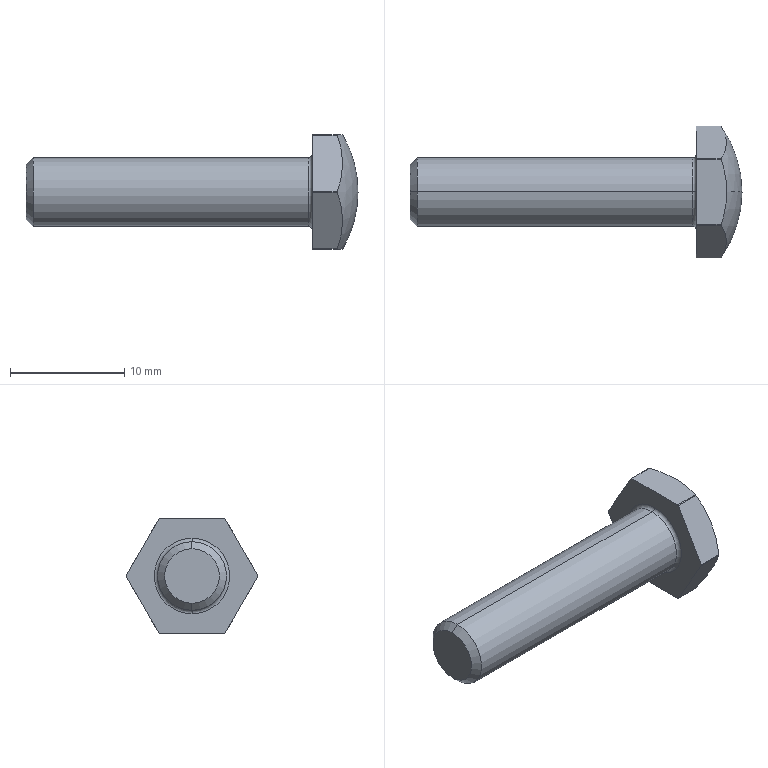Part | STEP file | SSTBB6-25-Part-1-2 | 1 solid | 22 faces | box 29 x 11.5 x 10 mm | volume 987.027 mm3 | cylinder 8 | plane 8 | cone 2 | torus 2 | sphere 2 | commonest cylinder face diameters 11.5 x6 6 x2
STEP:
#1=CARTESIAN_POINT('',(-5.,0.,2.387));
#2=VERTEX_POINT('',#1);
#3=CARTESIAN_POINT('',(-5.,0.,-2.387));
#4=VERTEX_POINT('',#3);
#5=CARTESIAN_POINT('',(-5.,0.,0.));
#6=DIRECTION('',(-1.,0.,0.));
#7=DIRECTION('',(0.,0.,1.));
#8=AXIS2_PLACEMENT_3D('',#5,#6,#7);
#9=CIRCLE('',#8,2.387);
#10=EDGE_CURVE('',#2,#4,#9,.T.);
#11=ORIENTED_EDGE('',*,*,#10,.F.);
#12=CARTESIAN_POINT('',(-4.386,0.,3.));
#13=VERTEX_POINT('',#12);
#14=CARTESIAN_POINT('',(-4.386,0.,3.));
#15=DIRECTION('',(0.7071,0.,0.7071));
#16=VECTOR('',#15,1000.);
#17=LINE('',#14,#16);
#18=EDGE_CURVE('',#2,#13,#17,.T.);
#19=ORIENTED_EDGE('',*,*,#18,.T.);
#20=CARTESIAN_POINT('',(-4.386,0.,-3.));
#21=VERTEX_POINT('',#20);
#22=CARTESIAN_POINT('',(-4.386,0.,0.));
#23=DIRECTION('',(-1.,0.,0.));
#24=DIRECTION('',(0.,0.,1.));
#25=AXIS2_PLACEMENT_3D('',#22,#23,#24);
#26=CIRCLE('',#25,3.);
#27=EDGE_CURVE('',#13,#21,#26,.T.);
#28=ORIENTED_EDGE('',*,*,#27,.T.);
#29=CARTESIAN_POINT('',(-4.386,0.,-3.));
#30=DIRECTION('',(0.7071,0.,-0.7071));
#31=VECTOR('',#30,1000.);
#32=LINE('',#29,#31);
#33=EDGE_CURVE('',#4,#21,#32,.T.);
#34=ORIENTED_EDGE('',*,*,#33,.F.);
#35=EDGE_LOOP('',(#11,#19,#28,#34));
#36=FACE_OUTER_BOUND('',#35,.T.);
#37=CARTESIAN_POINT('',(-4.386,0.,0.));
#38=DIRECTION('',(1.,0.,0.));
#39=DIRECTION('',(0.,0.,-1.));
#40=AXIS2_PLACEMENT_3D('',#37,#38,#39);
#41=CONICAL_SURFACE('',#40,3.,0.7854);
#42=ADVANCED_FACE('',(#36),#41,.T.);
#43=CARTESIAN_POINT('',(19.7,0.,3.));
#44=VERTEX_POINT('',#43);
#45=CARTESIAN_POINT('',(19.7,0.,-3.));
#46=VERTEX_POINT('',#45);
#47=CARTESIAN_POINT('',(19.7,0.,0.));
#48=DIRECTION('',(-1.,0.,0.));
#49=DIRECTION('',(0.,0.,1.));
#50=AXIS2_PLACEMENT_3D('',#47,#48,#49);
#51=CIRCLE('',#50,3.);
#52=EDGE_CURVE('',#44,#46,#51,.T.);
#53=ORIENTED_EDGE('',*,*,#52,.T.);
#54=CARTESIAN_POINT('',(0.,0.,-3.));
#55=DIRECTION('',(-1.,0.,0.));
#56=VECTOR('',#55,1000.);
#57=LINE('',#54,#56);
#58=EDGE_CURVE('',#46,#21,#57,.T.);
#59=ORIENTED_EDGE('',*,*,#58,.T.);
#60=ORIENTED_EDGE('',*,*,#27,.F.);
#61=CARTESIAN_POINT('',(0.,0.,3.));
#62=DIRECTION('',(-1.,0.,0.));
#63=VECTOR('',#62,1000.);
#64=LINE('',#61,#63);
#65=EDGE_CURVE('',#44,#13,#64,.T.);
#66=ORIENTED_EDGE('',*,*,#65,.F.);
#67=EDGE_LOOP('',(#53,#59,#60,#66));
#68=FACE_OUTER_BOUND('',#67,.T.);
#69=CARTESIAN_POINT('',(0.,0.,0.));
#70=DIRECTION('',(-1.,0.,0.));
#71=DIRECTION('',(0.,0.,1.));
#72=AXIS2_PLACEMENT_3D('',#69,#70,#71);
#73=CYLINDRICAL_SURFACE('',#72,3.);
#74=ADVANCED_FACE('',(#68),#73,.T.);
#75=CARTESIAN_POINT('',(19.7,0.,0.));
#76=DIRECTION('',(-1.,0.,0.));
#77=DIRECTION('',(0.,0.,1.));
#78=AXIS2_PLACEMENT_3D('',#75,#76,#77);
#79=CIRCLE('',#78,3.);
#80=EDGE_CURVE('',#46,#44,#79,.T.);
#81=ORIENTED_EDGE('',*,*,#80,.F.);
#82=CARTESIAN_POINT('',(20.,0.,-3.3));
#83=VERTEX_POINT('',#82);
#84=CARTESIAN_POINT('',(19.7,0.,-3.3));
#85=DIRECTION('',(0.,1.,0.));
#86=DIRECTION('',(0.,0.,1.));
#87=AXIS2_PLACEMENT_3D('',#84,#85,#86);
#88=CIRCLE('',#87,0.3);
#89=EDGE_CURVE('',#46,#83,#88,.T.);
#90=ORIENTED_EDGE('',*,*,#89,.T.);
#91=CARTESIAN_POINT('',(20.,0.,3.3));
#92=VERTEX_POINT('',#91);
#93=CARTESIAN_POINT('',(20.,0.,0.));
#94=DIRECTION('',(-1.,0.,0.));
#95=DIRECTION('',(0.,0.,1.));
#96=AXIS2_PLACEMENT_3D('',#93,#94,#95);
#97=CIRCLE('',#96,3.3);
#98=EDGE_CURVE('',#83,#92,#97,.T.);
#99=ORIENTED_EDGE('',*,*,#98,.T.);
#100=CARTESIAN_POINT('',(19.7,0.,3.3));
#101=DIRECTION('',(0.,-1.,0.));
#102=DIRECTION('',(0.,0.,-1.));
#103=AXIS2_PLACEMENT_3D('',#100,#101,#102);
#104=CIRCLE('',#103,0.3);
#105=EDGE_CURVE('',#44,#92,#104,.T.);
#106=ORIENTED_EDGE('',*,*,#105,.F.);
#107=EDGE_LOOP('',(#81,#90,#99,#106));
#108=FACE_OUTER_BOUND('',#107,.T.);
#109=CARTESIAN_POINT('',(19.7,0.,0.));
#110=DIRECTION('',(-1.,0.,0.));
#111=DIRECTION('',(0.,0.,1.));
#112=AXIS2_PLACEMENT_3D('',#109,#110,#111);
#113=TOROIDAL_SURFACE('',#112,3.3,0.3);
#114=ADVANCED_FACE('',(#108),#113,.F.);
#115=CARTESIAN_POINT('',(24.,0.,0.));
#116=VERTEX_POINT('',#115);
#117=CARTESIAN_POINT('',(22.66,0.,5.));
#118=VERTEX_POINT('',#117);
#119=CARTESIAN_POINT('',(14.,0.,0.));
#120=DIRECTION('',(0.,-1.,0.));
#121=DIRECTION('',(0.,0.,-1.));
#122=AXIS2_PLACEMENT_3D('',#119,#120,#121);
#123=CIRCLE('',#122,10.);
#124=EDGE_CURVE('',#116,#118,#123,.T.);
#125=ORIENTED_EDGE('',*,*,#124,.F.);
#126=CARTESIAN_POINT('',(22.66,0.,-5.));
#127=VERTEX_POINT('',#126);
#128=CARTESIAN_POINT('',(14.,0.,0.));
#129=DIRECTION('',(0.,1.,0.));
#130=DIRECTION('',(0.,0.,1.));
#131=AXIS2_PLACEMENT_3D('',#128,#129,#130);
#132=CIRCLE('',#131,10.);
#133=EDGE_CURVE('',#116,#127,#132,.T.);
#134=ORIENTED_EDGE('',*,*,#133,.T.);
#135=CARTESIAN_POINT('',(22.182,2.839,-5.));
#136=VERTEX_POINT('',#135);
#137=CARTESIAN_POINT('',(14.,0.,-5.));
#138=DIRECTION('',(0.,0.,1.));
#139=DIRECTION('',(-1.,0.,0.));
#140=AXIS2_PLACEMENT_3D('',#137,#138,#139);
#141=CIRCLE('',#140,8.66);
#142=EDGE_CURVE('',#127,#136,#141,.T.);
#143=ORIENTED_EDGE('',*,*,#142,.T.);
#144=CARTESIAN_POINT('',(22.182,2.91,-4.959));
#145=VERTEX_POINT('',#144);
#146=CARTESIAN_POINT('',(22.182,0.,0.));
#147=DIRECTION('',(-1.,0.,0.));
#148=DIRECTION('',(0.,0.,1.));
#149=AXIS2_PLACEMENT_3D('',#146,#147,#148);
#150=CIRCLE('',#149,5.75);
#151=EDGE_CURVE('',#145,#136,#150,.T.);
#152=ORIENTED_EDGE('',*,*,#151,.F.);
#153=CARTESIAN_POINT('',(22.182,5.75,-0.04096));
#154=VERTEX_POINT('',#153);
#155=CARTESIAN_POINT('',(14.,4.33,-2.5));
#156=DIRECTION('',(0.,-0.866,0.5));
#157=DIRECTION('',(0.,-0.5,-0.866));
#158=AXIS2_PLACEMENT_3D('',#155,#156,#157);
#159=CIRCLE('',#158,8.66);
#160=EDGE_CURVE('',#145,#154,#159,.T.);
#161=ORIENTED_EDGE('',*,*,#160,.T.);
#162=CARTESIAN_POINT('',(22.182,5.75,0.04096));
#163=VERTEX_POINT('',#162);
#164=CARTESIAN_POINT('',(22.182,0.,0.));
#165=DIRECTION('',(-1.,0.,0.));
#166=DIRECTION('',(0.,0.,1.));
#167=AXIS2_PLACEMENT_3D('',#164,#165,#166);
#168=CIRCLE('',#167,5.75);
#169=EDGE_CURVE('',#163,#154,#168,.T.);
#170=ORIENTED_EDGE('',*,*,#169,.F.);
#171=CARTESIAN_POINT('',(22.182,2.91,4.959));
#172=VERTEX_POINT('',#171);
#173=CARTESIAN_POINT('',(14.,4.33,2.5));
#174=DIRECTION('',(0.,-0.866,-0.5));
#175=DIRECTION('',(0.,0.5,-0.866));
#176=AXIS2_PLACEMENT_3D('',#173,#174,#175);
#177=CIRCLE('',#176,8.66);
#178=EDGE_CURVE('',#163,#172,#177,.T.);
#179=ORIENTED_EDGE('',*,*,#178,.T.);
#180=CARTESIAN_POINT('',(22.182,2.839,5.));
#181=VERTEX_POINT('',#180);
#182=CARTESIAN_POINT('',(22.182,0.,0.));
#183=DIRECTION('',(-1.,0.,0.));
#184=DIRECTION('',(0.,0.,1.));
#185=AXIS2_PLACEMENT_3D('',#182,#183,#184);
#186=CIRCLE('',#185,5.75);
#187=EDGE_CURVE('',#181,#172,#186,.T.);
#188=ORIENTED_EDGE('',*,*,#187,.F.);
#189=CARTESIAN_POINT('',(14.,0.,5.));
#190=DIRECTION('',(0.,0.,-1.));
#191=DIRECTION('',(1.,0.,0.));
#192=AXIS2_PLACEMENT_3D('',#189,#190,#191);
#193=CIRCLE('',#192,8.66);
#194=EDGE_CURVE('',#181,#118,#193,.T.);
#195=ORIENTED_EDGE('',*,*,#194,.T.);
#196=EDGE_LOOP('',(#125,#134,#143,#152,#161,#170,#179,#188,#195));
#197=FACE_OUTER_BOUND('',#196,.T.);
#198=CARTESIAN_POINT('',(14.,0.,0.));
#199=DIRECTION('',(0.,1.,0.));
#200=DIRECTION('',(0.,0.,1.));
#201=AXIS2_PLACEMENT_3D('',#198,#199,#200);
#202=SPHERICAL_SURFACE('',#201,10.);
#203=ADVANCED_FACE('',(#197),#202,.T.);
#204=ORIENTED_EDGE('',*,*,#133,.F.);
#205=ORIENTED_EDGE('',*,*,#124,.T.);
#206=CARTESIAN_POINT('',(22.182,-2.839,5.));
#207=VERTEX_POINT('',#206);
#208=CARTESIAN_POINT('',(14.,0.,5.));
#209=DIRECTION('',(0.,0.,-1.));
#210=DIRECTION('',(1.,0.,0.));
#211=AXIS2_PLACEMENT_3D('',#208,#209,#210);
#212=CIRCLE('',#211,8.66);
#213=EDGE_CURVE('',#118,#207,#212,.T.);
#214=ORIENTED_EDGE('',*,*,#213,.T.);
#215=CARTESIAN_POINT('',(22.182,-2.91,4.959));
#216=VERTEX_POINT('',#215);
#217=CARTESIAN_POINT('',(22.182,0.,0.));
#218=DIRECTION('',(-1.,0.,0.));
#219=DIRECTION('',(0.,0.,1.));
#220=AXIS2_PLACEMENT_3D('',#217,#218,#219);
#221=CIRCLE('',#220,5.75);
#222=EDGE_CURVE('',#216,#207,#221,.T.);
#223=ORIENTED_EDGE('',*,*,#222,.F.);
#224=CARTESIAN_POINT('',(22.182,-5.75,0.04096));
#225=VERTEX_POINT('',#224);
#226=CARTESIAN_POINT('',(14.,-4.33,2.5));
#227=DIRECTION('',(0.,0.866,-0.5));
#228=DIRECTION('',(0.,0.5,0.866));
#229=AXIS2_PLACEMENT_3D('',#226,#227,#228);
#230=CIRCLE('',#229,8.66);
#231=EDGE_CURVE('',#216,#225,#230,.T.);
#232=ORIENTED_EDGE('',*,*,#231,.T.);
#233=CARTESIAN_POINT('',(22.182,-5.75,-0.04096));
#234=VERTEX_POINT('',#233);
#235=CARTESIAN_POINT('',(22.182,0.,0.));
#236=DIRECTION('',(-1.,0.,0.));
#237=DIRECTION('',(0.,0.,1.));
#238=AXIS2_PLACEMENT_3D('',#235,#236,#237);
#239=CIRCLE('',#238,5.75);
#240=EDGE_CURVE('',#234,#225,#239,.T.);
#241=ORIENTED_EDGE('',*,*,#240,.F.);
#242=CARTESIAN_POINT('',(22.182,-2.91,-4.959));
#243=VERTEX_POINT('',#242);
#244=CARTESIAN_POINT('',(14.,-4.33,-2.5));
#245=DIRECTION('',(0.,0.866,0.5));
#246=DIRECTION('',(0.,-0.5,0.866));
#247=AXIS2_PLACEMENT_3D('',#244,#245,#246);
#248=CIRCLE('',#247,8.66);
#249=EDGE_CURVE('',#234,#243,#248,.T.);
#250=ORIENTED_EDGE('',*,*,#249,.T.);
#251=CARTESIAN_POINT('',(22.182,-2.839,-5.));
#252=VERTEX_POINT('',#251);
#253=CARTESIAN_POINT('',(22.182,0.,0.));
#254=DIRECTION('',(-1.,0.,0.));
#255=DIRECTION('',(0.,0.,1.));
#256=AXIS2_PLACEMENT_3D('',#253,#254,#255);
#257=CIRCLE('',#256,5.75);
#258=EDGE_CURVE('',#252,#243,#257,.T.);
#259=ORIENTED_EDGE('',*,*,#258,.F.);
#260=CARTESIAN_POINT('',(14.,0.,-5.));
#261=DIRECTION('',(0.,0.,1.));
#262=DIRECTION('',(-1.,0.,0.));
#263=AXIS2_PLACEMENT_3D('',#260,#261,#262);
#264=CIRCLE('',#263,8.66);
#265=EDGE_CURVE('',#252,#127,#264,.T.);
#266=ORIENTED_EDGE('',*,*,#265,.T.);
#267=EDGE_LOOP('',(#204,#205,#214,#223,#232,#241,#250,#259,#266));
#268=FACE_OUTER_BOUND('',#267,.T.);
#269=CARTESIAN_POINT('',(14.,0.,0.));
#270=DIRECTION('',(0.,1.,0.));
#271=DIRECTION('',(0.,0.,1.));
#272=AXIS2_PLACEMENT_3D('',#269,#270,#271);
#273=SPHERICAL_SURFACE('',#272,10.);
#274=ADVANCED_FACE('',(#268),#273,.T.);
#275=CARTESIAN_POINT('',(20.,-2.839,-5.));
#276=VERTEX_POINT('',#275);
#277=CARTESIAN_POINT('',(0.,-2.839,-5.));
#278=DIRECTION('',(-1.,0.,0.));
#279=VECTOR('',#278,1000.);
#280=LINE('',#277,#279);
#281=EDGE_CURVE('',#252,#276,#280,.T.);
#282=ORIENTED_EDGE('',*,*,#281,.F.);
#283=ORIENTED_EDGE('',*,*,#258,.T.);
#284=CARTESIAN_POINT('',(20.,-2.91,-4.959));
#285=VERTEX_POINT('',#284);
#286=CARTESIAN_POINT('',(0.,-2.91,-4.959));
#287=DIRECTION('',(1.,0.,0.));
#288=VECTOR('',#287,1000.);
#289=LINE('',#286,#288);
#290=EDGE_CURVE('',#285,#243,#289,.T.);
#291=ORIENTED_EDGE('',*,*,#290,.F.);
#292=CARTESIAN_POINT('',(20.,0.,0.));
#293=DIRECTION('',(-1.,0.,0.));
#294=DIRECTION('',(0.,0.,1.));
#295=AXIS2_PLACEMENT_3D('',#292,#293,#294);
#296=CIRCLE('',#295,5.75);
#297=EDGE_CURVE('',#276,#285,#296,.T.);
#298=ORIENTED_EDGE('',*,*,#297,.F.);
#299=EDGE_LOOP('',(#282,#283,#291,#298));
#300=FACE_OUTER_BOUND('',#299,.T.);
#301=CARTESIAN_POINT('',(0.,0.,0.));
#302=DIRECTION('',(-1.,0.,0.));
#303=DIRECTION('',(0.,0.,1.));
#304=AXIS2_PLACEMENT_3D('',#301,#302,#303);
#305=CYLINDRICAL_SURFACE('',#304,5.75);
#306=ADVANCED_FACE('',(#300),#305,.T.);
#307=CARTESIAN_POINT('',(20.,2.839,-5.));
#308=VERTEX_POINT('',#307);
#309=CARTESIAN_POINT('',(0.,2.839,-5.));
#310=DIRECTION('',(1.,0.,0.));
#311=VECTOR('',#310,1000.);
#312=LINE('',#309,#311);
#313=EDGE_CURVE('',#308,#136,#312,.T.);
#314=ORIENTED_EDGE('',*,*,#313,.F.);
#315=CARTESIAN_POINT('',(20.,2.91,-4.959));
#316=VERTEX_POINT('',#315);
#317=CARTESIAN_POINT('',(20.,0.,0.));
#318=DIRECTION('',(-1.,0.,0.));
#319=DIRECTION('',(0.,0.,1.));
#320=AXIS2_PLACEMENT_3D('',#317,#318,#319);
#321=CIRCLE('',#320,5.75);
#322=EDGE_CURVE('',#316,#308,#321,.T.);
#323=ORIENTED_EDGE('',*,*,#322,.F.);
#324=CARTESIAN_POINT('',(0.,2.91,-4.959));
#325=DIRECTION('',(-1.,0.,0.));
#326=VECTOR('',#325,1000.);
#327=LINE('',#324,#326);
#328=EDGE_CURVE('',#145,#316,#327,.T.);
#329=ORIENTED_EDGE('',*,*,#328,.F.);
#330=ORIENTED_EDGE('',*,*,#151,.T.);
#331=EDGE_LOOP('',(#314,#323,#329,#330));
#332=FACE_OUTER_BOUND('',#331,.T.);
#333=CARTESIAN_POINT('',(0.,0.,0.));
#334=DIRECTION('',(-1.,0.,0.));
#335=DIRECTION('',(0.,0.,1.));
#336=AXIS2_PLACEMENT_3D('',#333,#334,#335);
#337=CYLINDRICAL_SURFACE('',#336,5.75);
#338=ADVANCED_FACE('',(#332),#337,.T.);
#339=CARTESIAN_POINT('',(20.,5.75,-0.04096));
#340=VERTEX_POINT('',#339);
#341=CARTESIAN_POINT('',(0.,5.75,-0.04096));
#342=DIRECTION('',(1.,0.,0.));
#343=VECTOR('',#342,1000.);
#344=LINE('',#341,#343);
#345=EDGE_CURVE('',#340,#154,#344,.T.);
#346=ORIENTED_EDGE('',*,*,#345,.F.);
#347=CARTESIAN_POINT('',(20.,5.75,0.04096));
#348=VERTEX_POINT('',#347);
#349=CARTESIAN_POINT('',(20.,0.,0.));
#350=DIRECTION('',(-1.,0.,0.));
#351=DIRECTION('',(0.,0.,1.));
#352=AXIS2_PLACEMENT_3D('',#349,#350,#351);
#353=CIRCLE('',#352,5.75);
#354=EDGE_CURVE('',#348,#340,#353,.T.);
#355=ORIENTED_EDGE('',*,*,#354,.F.);
#356=CARTESIAN_POINT('',(0.,5.75,0.04096));
#357=DIRECTION('',(-1.,0.,0.));
#358=VECTOR('',#357,1000.);
#359=LINE('',#356,#358);
#360=EDGE_CURVE('',#163,#348,#359,.T.);
#361=ORIENTED_EDGE('',*,*,#360,.F.);
#362=ORIENTED_EDGE('',*,*,#169,.T.);
#363=EDGE_LOOP('',(#346,#355,#361,#362));
#364=FACE_OUTER_BOUND('',#363,.T.);
#365=CARTESIAN_POINT('',(0.,0.,0.));
#366=DIRECTION('',(-1.,0.,0.));
#367=DIRECTION('',(0.,0.,1.));
#368=AXIS2_PLACEMENT_3D('',#365,#366,#367);
#369=CYLINDRICAL_SURFACE('',#368,5.75);
#370=ADVANCED_FACE('',(#364),#369,.T.);
#371=CARTESIAN_POINT('',(20.,2.91,4.959));
#372=VERTEX_POINT('',#371);
#373=CARTESIAN_POINT('',(0.,2.91,4.959));
#374=DIRECTION('',(1.,0.,0.));
#375=VECTOR('',#374,1000.);
#376=LINE('',#373,#375);
#377=EDGE_CURVE('',#372,#172,#376,.T.);
#378=ORIENTED_EDGE('',*,*,#377,.F.);
#379=CARTESIAN_POINT('',(20.,2.839,5.));
#380=VERTEX_POINT('',#379);
#381=CARTESIAN_POINT('',(20.,0.,0.));
#382=DIRECTION('',(-1.,0.,0.));
#383=DIRECTION('',(0.,0.,1.));
#384=AXIS2_PLACEMENT_3D('',#381,#382,#383);
#385=CIRCLE('',#384,5.75);
#386=EDGE_CURVE('',#380,#372,#385,.T.);
#387=ORIENTED_EDGE('',*,*,#386,.F.);
#388=CARTESIAN_POINT('',(0.,2.839,5.));
#389=DIRECTION('',(-1.,0.,0.));
#390=VECTOR('',#389,1000.);
#391=LINE('',#388,#390);
#392=EDGE_CURVE('',#181,#380,#391,.T.);
#393=ORIENTED_EDGE('',*,*,#392,.F.);
#394=ORIENTED_EDGE('',*,*,#187,.T.);
#395=EDGE_LOOP('',(#378,#387,#393,#394));
#396=FACE_OUTER_BOUND('',#395,.T.);
#397=CARTESIAN_POINT('',(0.,0.,0.));
#398=DIRECTION('',(-1.,0.,0.));
#399=DIRECTION('',(0.,0.,1.));
#400=AXIS2_PLACEMENT_3D('',#397,#398,#399);
#401=CYLINDRICAL_SURFACE('',#400,5.75);
#402=ADVANCED_FACE('',(#396),#401,.T.);
#403=CARTESIAN_POINT('',(20.,-2.839,5.));
#404=VERTEX_POINT('',#403);
#405=CARTESIAN_POINT('',(0.,-2.839,5.));
#406=DIRECTION('',(1.,0.,0.));
#407=VECTOR('',#406,1000.);
#408=LINE('',#405,#407);
#409=EDGE_CURVE('',#404,#207,#408,.T.);
#410=ORIENTED_EDGE('',*,*,#409,.F.);
#411=CARTESIAN_POINT('',(20.,-2.91,4.959));
#412=VERTEX_POINT('',#411);
#413=CARTESIAN_POINT('',(20.,0.,0.));
#414=DIRECTION('',(-1.,0.,0.));
#415=DIRECTION('',(0.,0.,1.));
#416=AXIS2_PLACEMENT_3D('',#413,#414,#415);
#417=CIRCLE('',#416,5.75);
#418=EDGE_CURVE('',#412,#404,#417,.T.);
#419=ORIENTED_EDGE('',*,*,#418,.F.);
#420=CARTESIAN_POINT('',(0.,-2.91,4.959));
#421=DIRECTION('',(-1.,0.,0.));
#422=VECTOR('',#421,1000.);
#423=LINE('',#420,#422);
#424=EDGE_CURVE('',#216,#412,#423,.T.);
#425=ORIENTED_EDGE('',*,*,#424,.F.);
#426=ORIENTED_EDGE('',*,*,#222,.T.);
#427=EDGE_LOOP('',(#410,#419,#425,#426));
#428=FACE_OUTER_BOUND('',#427,.T.);
#429=CARTESIAN_POINT('',(0.,0.,0.));
#430=DIRECTION('',(-1.,0.,0.));
#431=DIRECTION('',(0.,0.,1.));
#432=AXIS2_PLACEMENT_3D('',#429,#430,#431);
#433=CYLINDRICAL_SURFACE('',#432,5.75);
#434=ADVANCED_FACE('',(#428),#433,.T.);
#435=CARTESIAN_POINT('',(20.,-5.75,0.04096));
#436=VERTEX_POINT('',#435);
#437=CARTESIAN_POINT('',(0.,-5.75,0.04096));
#438=DIRECTION('',(1.,0.,0.));
#439=VECTOR('',#438,1000.);
#440=LINE('',#437,#439);
#441=EDGE_CURVE('',#436,#225,#440,.T.);
#442=ORIENTED_EDGE('',*,*,#441,.F.);
#443=CARTESIAN_POINT('',(20.,-5.75,-0.04096));
#444=VERTEX_POINT('',#443);
#445=CARTESIAN_POINT('',(20.,0.,0.));
#446=DIRECTION('',(-1.,0.,0.));
#447=DIRECTION('',(0.,0.,1.));
#448=AXIS2_PLACEMENT_3D('',#445,#446,#447);
#449=CIRCLE('',#448,5.75);
#450=EDGE_CURVE('',#444,#436,#449,.T.);
#451=ORIENTED_EDGE('',*,*,#450,.F.);
#452=CARTESIAN_POINT('',(0.,-5.75,-0.04096));
#453=DIRECTION('',(-1.,0.,0.));
#454=VECTOR('',#453,1000.);
#455=LINE('',#452,#454);
#456=EDGE_CURVE('',#234,#444,#455,.T.);
#457=ORIENTED_EDGE('',*,*,#456,.F.);
#458=ORIENTED_EDGE('',*,*,#240,.T.);
#459=EDGE_LOOP('',(#442,#451,#457,#458));
#460=FACE_OUTER_BOUND('',#459,.T.);
#461=CARTESIAN_POINT('',(0.,0.,0.));
#462=DIRECTION('',(-1.,0.,0.));
#463=DIRECTION('',(0.,0.,1.));
#464=AXIS2_PLACEMENT_3D('',#461,#462,#463);
#465=CYLINDRICAL_SURFACE('',#464,5.75);
#466=ADVANCED_FACE('',(#460),#465,.T.);
#467=CARTESIAN_POINT('',(20.,0.,0.));
#468=DIRECTION('',(-1.,0.,0.));
#469=DIRECTION('',(0.,0.,1.));
#470=AXIS2_PLACEMENT_3D('',#467,#468,#469);
#471=CIRCLE('',#470,3.3);
#472=EDGE_CURVE('',#92,#83,#471,.T.);
#473=ORIENTED_EDGE('',*,*,#472,.F.);
#474=ORIENTED_EDGE('',*,*,#98,.F.);
#475=EDGE_LOOP('',(#473,#474));
#476=FACE_BOUND('',#475,.T.);
#477=CARTESIAN_POINT('',(20.,0.,-5.));
#478=DIRECTION('',(0.,1.,0.));
#479=VECTOR('',#478,1000.);
#480=LINE('',#477,#479);
#481=EDGE_CURVE('',#276,#308,#480,.T.);
#482=ORIENTED_EDGE('',*,*,#481,.F.);
#483=ORIENTED_EDGE('',*,*,#297,.T.);
#484=CARTESIAN_POINT('',(20.,-6.82,1.812));
#485=DIRECTION('',(0.,0.5,-0.866));
#486=VECTOR('',#485,1000.);
#487=LINE('',#484,#486);
#488=EDGE_CURVE('',#444,#285,#487,.T.);
#489=ORIENTED_EDGE('',*,*,#488,.F.);
#490=ORIENTED_EDGE('',*,*,#450,.T.);
#491=CARTESIAN_POINT('',(20.,-1.84,6.812));
#492=DIRECTION('',(0.,-0.5,-0.866));
#493=VECTOR('',#492,1000.);
#494=LINE('',#491,#493);
#495=EDGE_CURVE('',#412,#436,#494,.T.);
#496=ORIENTED_EDGE('',*,*,#495,.F.);
#497=ORIENTED_EDGE('',*,*,#418,.T.);
#498=CARTESIAN_POINT('',(20.,0.,5.));
#499=DIRECTION('',(0.,-1.,0.));
#500=VECTOR('',#499,1000.);
#501=LINE('',#498,#500);
#502=EDGE_CURVE('',#380,#404,#501,.T.);
#503=ORIENTED_EDGE('',*,*,#502,.F.);
#504=ORIENTED_EDGE('',*,*,#386,.T.);
#505=CARTESIAN_POINT('',(20.,1.84,6.812));
#506=DIRECTION('',(0.,-0.5,0.866));
#507=VECTOR('',#506,1000.);
#508=LINE('',#505,#507);
#509=EDGE_CURVE('',#348,#372,#508,.T.);
#510=ORIENTED_EDGE('',*,*,#509,.F.);
#511=ORIENTED_EDGE('',*,*,#354,.T.);
#512=CARTESIAN_POINT('',(20.,6.82,1.812));
#513=DIRECTION('',(0.,0.5,0.866));
#514=VECTOR('',#513,1000.);
#515=LINE('',#512,#514);
#516=EDGE_CURVE('',#316,#340,#515,.T.);
#517=ORIENTED_EDGE('',*,*,#516,.F.);
#518=ORIENTED_EDGE('',*,*,#322,.T.);
#519=EDGE_LOOP('',(#482,#483,#489,#490,#496,#497,#503,#504,#510,#511,#517,#518));
#520=FACE_OUTER_BOUND('',#519,.T.);
#521=CARTESIAN_POINT('',(20.,0.,5.75));
#522=DIRECTION('',(1.,0.,0.));
#523=DIRECTION('',(0.,0.,-1.));
#524=AXIS2_PLACEMENT_3D('',#521,#522,#523);
#525=PLANE('',#524);
#526=ADVANCED_FACE('',(#476,#520),#525,.F.);
#527=ORIENTED_EDGE('',*,*,#89,.F.);
#528=ORIENTED_EDGE('',*,*,#52,.F.);
#529=ORIENTED_EDGE('',*,*,#105,.T.);
#530=ORIENTED_EDGE('',*,*,#472,.T.);
#531=EDGE_LOOP('',(#527,#528,#529,#530));
#532=FACE_OUTER_BOUND('',#531,.T.);
#533=CARTESIAN_POINT('',(19.7,0.,0.));
#534=DIRECTION('',(-1.,0.,0.));
#535=DIRECTION('',(0.,0.,1.));
#536=AXIS2_PLACEMENT_3D('',#533,#534,#535);
#537=TOROIDAL_SURFACE('',#536,3.3,0.3);
#538=ADVANCED_FACE('',(#532),#537,.F.);
#539=ORIENTED_EDGE('',*,*,#58,.F.);
#540=ORIENTED_EDGE('',*,*,#80,.T.);
#541=ORIENTED_EDGE('',*,*,#65,.T.);
#542=CARTESIAN_POINT('',(-4.386,0.,0.));
#543=DIRECTION('',(-1.,0.,0.));
#544=DIRECTION('',(0.,0.,1.));
#545=AXIS2_PLACEMENT_3D('',#542,#543,#544);
#546=CIRCLE('',#545,3.);
#547=EDGE_CURVE('',#21,#13,#546,.T.);
#548=ORIENTED_EDGE('',*,*,#547,.F.);
#549=EDGE_LOOP('',(#539,#540,#541,#548));
#550=FACE_OUTER_BOUND('',#549,.T.);
#551=CARTESIAN_POINT('',(0.,0.,0.));
#552=DIRECTION('',(-1.,0.,0.));
#553=DIRECTION('',(0.,0.,1.));
#554=AXIS2_PLACEMENT_3D('',#551,#552,#553);
#555=CYLINDRICAL_SURFACE('',#554,3.);
#556=ADVANCED_FACE('',(#550),#555,.T.);
#557=ORIENTED_EDGE('',*,*,#18,.F.);
#558=CARTESIAN_POINT('',(-5.,0.,0.));
#559=DIRECTION('',(-1.,0.,0.));
#560=DIRECTION('',(0.,0.,1.));
#561=AXIS2_PLACEMENT_3D('',#558,#559,#560);
#562=CIRCLE('',#561,2.387);
#563=EDGE_CURVE('',#4,#2,#562,.T.);
#564=ORIENTED_EDGE('',*,*,#563,.F.);
#565=ORIENTED_EDGE('',*,*,#33,.T.);
#566=ORIENTED_EDGE('',*,*,#547,.T.);
#567=EDGE_LOOP('',(#557,#564,#565,#566));
#568=FACE_OUTER_BOUND('',#567,.T.);
#569=CARTESIAN_POINT('',(-4.386,0.,0.));
#570=DIRECTION('',(1.,0.,0.));
#571=DIRECTION('',(0.,0.,-1.));
#572=AXIS2_PLACEMENT_3D('',#569,#570,#571);
#573=CONICAL_SURFACE('',#572,3.,0.7854);
#574=ADVANCED_FACE('',(#568),#573,.T.);
#575=ORIENTED_EDGE('',*,*,#563,.T.);
#576=ORIENTED_EDGE('',*,*,#10,.T.);
#577=EDGE_LOOP('',(#575,#576));
#578=FACE_OUTER_BOUND('',#577,.T.);
#579=CARTESIAN_POINT('',(-5.,0.,2.387));
#580=DIRECTION('',(1.,0.,0.));
#581=DIRECTION('',(0.,0.,-1.));
#582=AXIS2_PLACEMENT_3D('',#579,#580,#581);
#583=PLANE('',#582);
#584=ADVANCED_FACE('',(#578),#583,.F.);
#585=ORIENTED_EDGE('',*,*,#456,.T.);
#586=ORIENTED_EDGE('',*,*,#488,.T.);
#587=ORIENTED_EDGE('',*,*,#290,.T.);
#588=ORIENTED_EDGE('',*,*,#249,.F.);
#589=EDGE_LOOP('',(#585,#586,#587,#588));
#590=FACE_OUTER_BOUND('',#589,.T.);
#591=CARTESIAN_POINT('',(24.,-2.887,-5.));
#592=DIRECTION('',(0.,-0.866,-0.5));
#593=DIRECTION('',(0.,-0.5,0.866));
#594=AXIS2_PLACEMENT_3D('',#591,#592,#593);
#595=PLANE('',#594);
#596=ADVANCED_FACE('',(#590),#595,.T.);
#597=ORIENTED_EDGE('',*,*,#424,.T.);
#598=ORIENTED_EDGE('',*,*,#495,.T.);
#599=ORIENTED_EDGE('',*,*,#441,.T.);
#600=ORIENTED_EDGE('',*,*,#231,.F.);
#601=EDGE_LOOP('',(#597,#598,#599,#600));
#602=FACE_OUTER_BOUND('',#601,.T.);
#603=CARTESIAN_POINT('',(24.,-5.774,0.));
#604=DIRECTION('',(0.,-0.866,0.5));
#605=DIRECTION('',(0.,0.5,0.866));
#606=AXIS2_PLACEMENT_3D('',#603,#604,#605);
#607=PLANE('',#606);
#608=ADVANCED_FACE('',(#602),#607,.T.);
#609=ORIENTED_EDGE('',*,*,#392,.T.);
#610=ORIENTED_EDGE('',*,*,#502,.T.);
#611=ORIENTED_EDGE('',*,*,#409,.T.);
#612=ORIENTED_EDGE('',*,*,#213,.F.);
#613=ORIENTED_EDGE('',*,*,#194,.F.);
#614=EDGE_LOOP('',(#609,#610,#611,#612,#613));
#615=FACE_OUTER_BOUND('',#614,.T.);
#616=CARTESIAN_POINT('',(24.,-2.887,5.));
#617=DIRECTION('',(0.,0.,1.));
#618=DIRECTION('',(1.,0.,0.));
#619=AXIS2_PLACEMENT_3D('',#616,#617,#618);
#620=PLANE('',#619);
#621=ADVANCED_FACE('',(#615),#620,.T.);
#622=ORIENTED_EDGE('',*,*,#360,.T.);
#623=ORIENTED_EDGE('',*,*,#509,.T.);
#624=ORIENTED_EDGE('',*,*,#377,.T.);
#625=ORIENTED_EDGE('',*,*,#178,.F.);
#626=EDGE_LOOP('',(#622,#623,#624,#625));
#627=FACE_OUTER_BOUND('',#626,.T.);
#628=CARTESIAN_POINT('',(24.,2.887,5.));
#629=DIRECTION('',(0.,0.866,0.5));
#630=DIRECTION('',(0.,0.5,-0.866));
#631=AXIS2_PLACEMENT_3D('',#628,#629,#630);
#632=PLANE('',#631);
#633=ADVANCED_FACE('',(#627),#632,.T.);
#634=ORIENTED_EDGE('',*,*,#328,.T.);
#635=ORIENTED_EDGE('',*,*,#516,.T.);
#636=ORIENTED_EDGE('',*,*,#345,.T.);
#637=ORIENTED_EDGE('',*,*,#160,.F.);
#638=EDGE_LOOP('',(#634,#635,#636,#637));
#639=FACE_OUTER_BOUND('',#638,.T.);
#640=CARTESIAN_POINT('',(24.,5.774,0.));
#641=DIRECTION('',(0.,0.866,-0.5));
#642=DIRECTION('',(0.,-0.5,-0.866));
#643=AXIS2_PLACEMENT_3D('',#640,#641,#642);
#644=PLANE('',#643);
#645=ADVANCED_FACE('',(#639),#644,.T.);
#646=ORIENTED_EDGE('',*,*,#281,.T.);
#647=ORIENTED_EDGE('',*,*,#481,.T.);
#648=ORIENTED_EDGE('',*,*,#313,.T.);
#649=ORIENTED_EDGE('',*,*,#142,.F.);
#650=ORIENTED_EDGE('',*,*,#265,.F.);
#651=EDGE_LOOP('',(#646,#647,#648,#649,#650));
#652=FACE_OUTER_BOUND('',#651,.T.);
#653=CARTESIAN_POINT('',(24.,2.887,-5.));
#654=DIRECTION('',(0.,0.,-1.));
#655=DIRECTION('',(-1.,0.,0.));
#656=AXIS2_PLACEMENT_3D('',#653,#654,#655);
#657=PLANE('',#656);
#658=ADVANCED_FACE('',(#652),#657,.T.);
#659=CLOSED_SHELL('',(#42,#74,#114,#203,#274,#306,#338,#370,#402,#434,#466,#526,#538,#556,#574,#584,#596,#608,#621,#633,#645,#658));
#660=MANIFOLD_SOLID_BREP('',#659);
#661=CARTESIAN_POINT('',(0.,0.,0.));
#662=DIRECTION('',(0.,0.,1.));
#663=DIRECTION('',(1.,0.,0.));
#664=AXIS2_PLACEMENT_3D('',#661,#662,#663);
#665=(LENGTH_UNIT()NAMED_UNIT(*)SI_UNIT(.MILLI.,.METRE.));
#666=UNCERTAINTY_MEASURE_WITH_UNIT(LENGTH_MEASURE(0.00001),#665,'','');
#667=(NAMED_UNIT(*)PLANE_ANGLE_UNIT()SI_UNIT($,.RADIAN.));
#668=(NAMED_UNIT(*)SI_UNIT($,.STERADIAN.)SOLID_ANGLE_UNIT());
#669=(GEOMETRIC_REPRESENTATION_CONTEXT(3)GLOBAL_UNCERTAINTY_ASSIGNED_CONTEXT((#666))GLOBAL_UNIT_ASSIGNED_CONTEXT((#665,#667,#668))REPRESENTATION_CONTEXT('',''));
#670=ADVANCED_BREP_SHAPE_REPRESENTATION('',(#660,#664),#669);